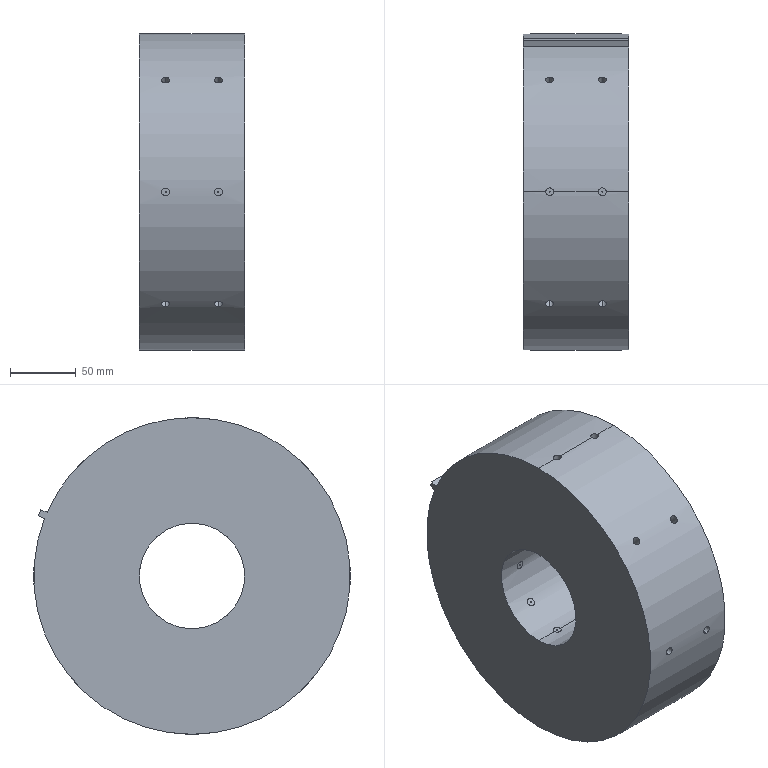Part | SolidWorks | features ICE 4, CirPattern 1, Extrusion 1, MirrorPattern 1 | 1 solid | 138 faces | box 80 x 240 x 240 mm | volume 3186685 mm3 | cylinder 101 | plane 37 | commonest cylinder face diameters 6 x64 0.6 x32 240 x3 80.06 x2